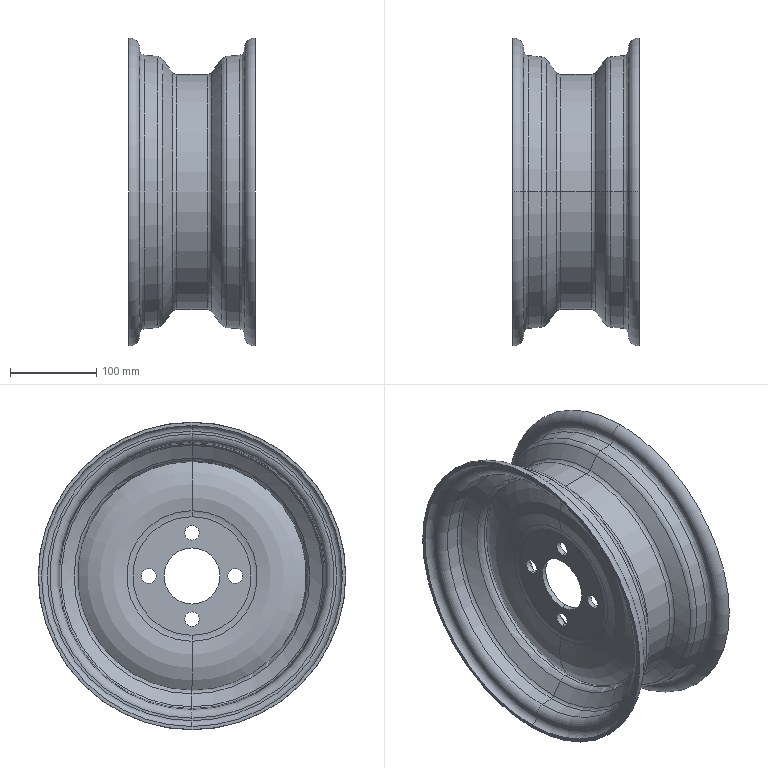Part | SolidWorks | features ICE 1, Revolution 1 | 1 solid | 83 faces | box 146.265 x 355.938 x 355.938 mm | volume 972609 mm3 | torus 42 | cylinder 16 | cone 16 | plane 9 | commonest cylinder face diameters 17 x8 65 x2 254.396 x2 265.027 x2 272.196 x2